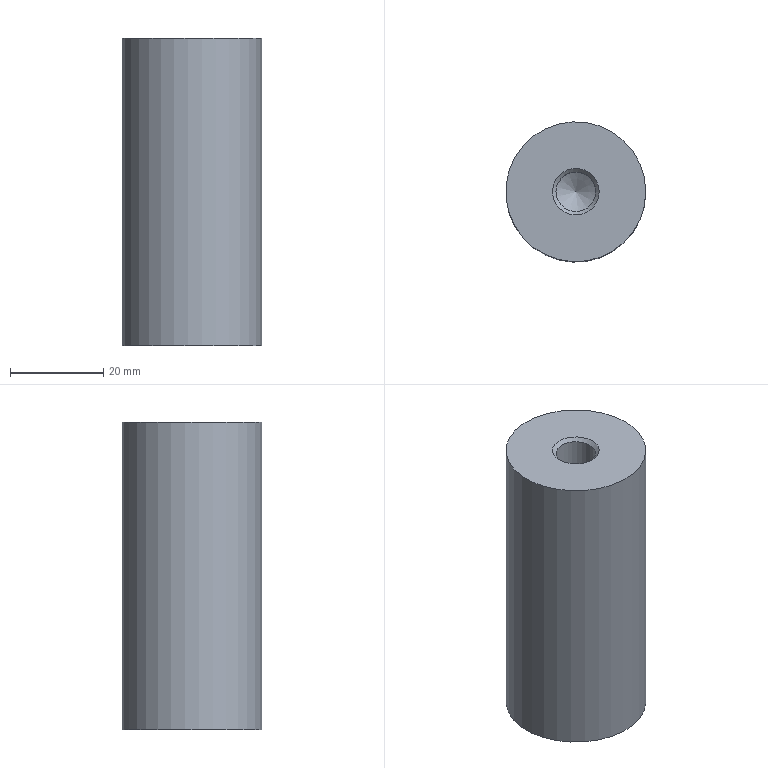Part | NX | features DATUM_CSYS 2, HOLE PACKAGE 2, SIMPLE HOLE 2, SYMBOLIC_THREAD 2, EXTRUDE 1, SKETCH 1 | 1 solid | 9 faces | box 30 x 30 x 66 mm | volume 43249 mm3 | cone 4 | cylinder 3 | plane 2 | commonest cylinder face diameters 8.5 x2 30 x1
STEP:
#1=CARTESIAN_POINT('',(15.,0.,66.));
#2=VERTEX_POINT('',#1);
#3=CARTESIAN_POINT('',(0.,0.,66.));
#4=DIRECTION('',(0.,0.,1.));
#5=DIRECTION('',(1.,0.,0.));
#6=AXIS2_PLACEMENT_3D('',#3,#4,#5);
#7=CIRCLE('',#6,15.);
#8=EDGE_CURVE('',#2,#2,#7,.T.);
#9=ORIENTED_EDGE('',*,*,#8,.F.);
#10=EDGE_LOOP('',(#9));
#11=FACE_BOUND('',#10,.T.);
#12=CARTESIAN_POINT('',(15.,0.,0.));
#13=VERTEX_POINT('',#12);
#14=CARTESIAN_POINT('',(0.,0.,0.));
#15=DIRECTION('',(0.,0.,1.));
#16=DIRECTION('',(1.,0.,0.));
#17=AXIS2_PLACEMENT_3D('',#14,#15,#16);
#18=CIRCLE('',#17,15.);
#19=EDGE_CURVE('',#13,#13,#18,.T.);
#20=ORIENTED_EDGE('',*,*,#19,.T.);
#21=EDGE_LOOP('',(#20));
#22=FACE_BOUND('',#21,.T.);
#23=CARTESIAN_POINT('',(0.,0.,66.));
#24=DIRECTION('',(0.,0.,-1.));
#25=DIRECTION('',(-1.,0.,0.));
#26=AXIS2_PLACEMENT_3D('',#23,#24,#25);
#27=CYLINDRICAL_SURFACE('',#26,15.);
#28=ADVANCED_FACE('',(#11,#22),#27,.T.);
#29=CARTESIAN_POINT('',(5.,0.,66.));
#30=VERTEX_POINT('',#29);
#31=CARTESIAN_POINT('',(0.,0.,66.));
#32=DIRECTION('',(0.,0.,1.));
#33=DIRECTION('',(1.,0.,0.));
#34=AXIS2_PLACEMENT_3D('',#31,#32,#33);
#35=CIRCLE('',#34,5.);
#36=EDGE_CURVE('',#30,#30,#35,.T.);
#37=ORIENTED_EDGE('',*,*,#36,.F.);
#38=EDGE_LOOP('',(#37));
#39=FACE_BOUND('',#38,.T.);
#40=ORIENTED_EDGE('',*,*,#8,.T.);
#41=EDGE_LOOP('',(#40));
#42=FACE_BOUND('',#41,.T.);
#43=CARTESIAN_POINT('',(0.,0.,66.));
#44=DIRECTION('',(0.,0.,1.));
#45=DIRECTION('',(1.,0.,0.));
#46=AXIS2_PLACEMENT_3D('',#43,#44,#45);
#47=PLANE('',#46);
#48=ADVANCED_FACE('',(#39,#42),#47,.T.);
#49=CARTESIAN_POINT('',(5.,0.,0.));
#50=VERTEX_POINT('',#49);
#51=CARTESIAN_POINT('',(0.,0.,0.));
#52=DIRECTION('',(0.,0.,1.));
#53=DIRECTION('',(1.,0.,0.));
#54=AXIS2_PLACEMENT_3D('',#51,#52,#53);
#55=CIRCLE('',#54,5.);
#56=EDGE_CURVE('',#50,#50,#55,.T.);
#57=ORIENTED_EDGE('',*,*,#56,.T.);
#58=EDGE_LOOP('',(#57));
#59=FACE_BOUND('',#58,.T.);
#60=ORIENTED_EDGE('',*,*,#19,.F.);
#61=EDGE_LOOP('',(#60));
#62=FACE_BOUND('',#61,.T.);
#63=CARTESIAN_POINT('',(0.,0.,0.));
#64=DIRECTION('',(0.,0.,1.));
#65=DIRECTION('',(1.,0.,0.));
#66=AXIS2_PLACEMENT_3D('',#63,#64,#65);
#67=PLANE('',#66);
#68=ADVANCED_FACE('',(#59,#62),#67,.F.);
#69=ORIENTED_EDGE('',*,*,#36,.T.);
#70=EDGE_LOOP('',(#69));
#71=FACE_BOUND('',#70,.T.);
#72=CARTESIAN_POINT('',(4.25,0.,65.25));
#73=VERTEX_POINT('',#72);
#74=CARTESIAN_POINT('',(0.,0.,65.25));
#75=DIRECTION('',(0.,0.,1.));
#76=DIRECTION('',(1.,0.,0.));
#77=AXIS2_PLACEMENT_3D('',#74,#75,#76);
#78=CIRCLE('',#77,4.25);
#79=EDGE_CURVE('',#73,#73,#78,.T.);
#80=ORIENTED_EDGE('',*,*,#79,.F.);
#81=EDGE_LOOP('',(#80));
#82=FACE_BOUND('',#81,.T.);
#83=CARTESIAN_POINT('',(0.,0.,61.));
#84=DIRECTION('',(0.,0.,1.));
#85=DIRECTION('',(1.,0.,0.));
#86=AXIS2_PLACEMENT_3D('',#83,#84,#85);
#87=CONICAL_SURFACE('',#86,0.,0.7854);
#88=ADVANCED_FACE('',(#71,#82),#87,.F.);
#89=CARTESIAN_POINT('',(-4.25,0.,38.5));
#90=VERTEX_POINT('',#89);
#91=CARTESIAN_POINT('',(0.,0.,38.5));
#92=DIRECTION('',(0.,0.,-1.));
#93=DIRECTION('',(-1.,0.,0.));
#94=AXIS2_PLACEMENT_3D('',#91,#92,#93);
#95=CIRCLE('',#94,4.25);
#96=EDGE_CURVE('',#90,#90,#95,.F.);
#97=ORIENTED_EDGE('',*,*,#96,.T.);
#98=EDGE_LOOP('',(#97));
#99=FACE_BOUND('',#98,.T.);
#100=CARTESIAN_POINT('',(0.,0.,35.946));
#101=VERTEX_POINT('',#100);
#102=VERTEX_LOOP('',#101);
#103=FACE_BOUND('',#102,.T.);
#104=CARTESIAN_POINT('',(0.,0.,38.5));
#105=DIRECTION('',(0.,0.,1.));
#106=DIRECTION('',(1.,0.,0.));
#107=AXIS2_PLACEMENT_3D('',#104,#105,#106);
#108=CONICAL_SURFACE('',#107,4.25,1.03);
#109=ADVANCED_FACE('',(#99,#103),#108,.F.);
#110=ORIENTED_EDGE('',*,*,#79,.T.);
#111=EDGE_LOOP('',(#110));
#112=FACE_BOUND('',#111,.T.);
#113=ORIENTED_EDGE('',*,*,#96,.F.);
#114=EDGE_LOOP('',(#113));
#115=FACE_BOUND('',#114,.T.);
#116=CARTESIAN_POINT('',(0.,0.,66.));
#117=DIRECTION('',(0.,0.,-1.));
#118=DIRECTION('',(-1.,0.,0.));
#119=AXIS2_PLACEMENT_3D('',#116,#117,#118);
#120=CYLINDRICAL_SURFACE('',#119,4.25);
#121=ADVANCED_FACE('',(#112,#115),#120,.F.);
#122=CARTESIAN_POINT('',(-4.25,0.,0.75));
#123=VERTEX_POINT('',#122);
#124=CARTESIAN_POINT('',(0.,0.,0.75));
#125=DIRECTION('',(0.,0.,-1.));
#126=DIRECTION('',(-1.,0.,0.));
#127=AXIS2_PLACEMENT_3D('',#124,#125,#126);
#128=CIRCLE('',#127,4.25);
#129=EDGE_CURVE('',#123,#123,#128,.T.);
#130=ORIENTED_EDGE('',*,*,#129,.F.);
#131=EDGE_LOOP('',(#130));
#132=FACE_BOUND('',#131,.T.);
#133=ORIENTED_EDGE('',*,*,#56,.F.);
#134=EDGE_LOOP('',(#133));
#135=FACE_BOUND('',#134,.T.);
#136=CARTESIAN_POINT('',(0.,0.,5.));
#137=DIRECTION('',(0.,0.,-1.));
#138=DIRECTION('',(-1.,0.,0.));
#139=AXIS2_PLACEMENT_3D('',#136,#137,#138);
#140=CONICAL_SURFACE('',#139,0.,0.7854);
#141=ADVANCED_FACE('',(#132,#135),#140,.F.);
#142=CARTESIAN_POINT('',(4.25,0.,30.5));
#143=VERTEX_POINT('',#142);
#144=CARTESIAN_POINT('',(0.,0.,30.5));
#145=DIRECTION('',(0.,0.,1.));
#146=DIRECTION('',(1.,0.,0.));
#147=AXIS2_PLACEMENT_3D('',#144,#145,#146);
#148=CIRCLE('',#147,4.25);
#149=EDGE_CURVE('',#143,#143,#148,.F.);
#150=ORIENTED_EDGE('',*,*,#149,.T.);
#151=EDGE_LOOP('',(#150));
#152=FACE_BOUND('',#151,.T.);
#153=CARTESIAN_POINT('',(0.,0.,33.054));
#154=VERTEX_POINT('',#153);
#155=VERTEX_LOOP('',#154);
#156=FACE_BOUND('',#155,.T.);
#157=CARTESIAN_POINT('',(0.,0.,30.5));
#158=DIRECTION('',(0.,0.,-1.));
#159=DIRECTION('',(-1.,0.,0.));
#160=AXIS2_PLACEMENT_3D('',#157,#158,#159);
#161=CONICAL_SURFACE('',#160,4.25,1.03);
#162=ADVANCED_FACE('',(#152,#156),#161,.F.);
#163=ORIENTED_EDGE('',*,*,#129,.T.);
#164=EDGE_LOOP('',(#163));
#165=FACE_BOUND('',#164,.T.);
#166=ORIENTED_EDGE('',*,*,#149,.F.);
#167=EDGE_LOOP('',(#166));
#168=FACE_BOUND('',#167,.T.);
#169=CARTESIAN_POINT('',(0.,0.,0.));
#170=DIRECTION('',(0.,0.,1.));
#171=DIRECTION('',(1.,0.,0.));
#172=AXIS2_PLACEMENT_3D('',#169,#170,#171);
#173=CYLINDRICAL_SURFACE('',#172,4.25);
#174=ADVANCED_FACE('',(#165,#168),#173,.F.);
#175=CLOSED_SHELL('',(#28,#48,#68,#88,#109,#121,#141,#162,#174));
#176=MANIFOLD_SOLID_BREP('',#175);
#177=(LENGTH_UNIT()NAMED_UNIT(*)SI_UNIT(.MILLI.,.METRE.));
#178=UNCERTAINTY_MEASURE_WITH_UNIT(LENGTH_MEASURE(0.00001),#177,'','');
#179=(NAMED_UNIT(*)PLANE_ANGLE_UNIT()SI_UNIT($,.RADIAN.));
#180=(NAMED_UNIT(*)SI_UNIT($,.STERADIAN.)SOLID_ANGLE_UNIT());
#181=(GEOMETRIC_REPRESENTATION_CONTEXT(3)GLOBAL_UNCERTAINTY_ASSIGNED_CONTEXT((#178))GLOBAL_UNIT_ASSIGNED_CONTEXT((#177,#179,#180))REPRESENTATION_CONTEXT('',''));
#182=ADVANCED_BREP_SHAPE_REPRESENTATION('',(#176),#181);